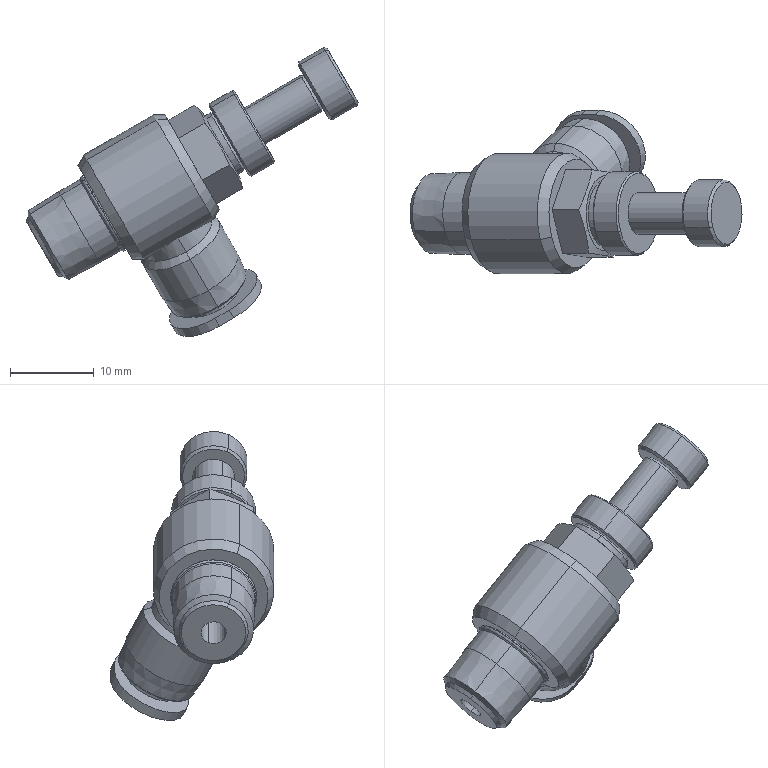Part | NX | features J-XZB01-D6-1.SLDPRT 2 | 1 solid | 84 faces | box 39.672 x 19.542 x 34.537 mm | volume 4093 mm3 | cone 32 | cylinder 28 | plane 22 | torus 2 | commonest cylinder face diameters 9.8 x6 8 x4 3 x2 5 x2 6 x2 7 x2